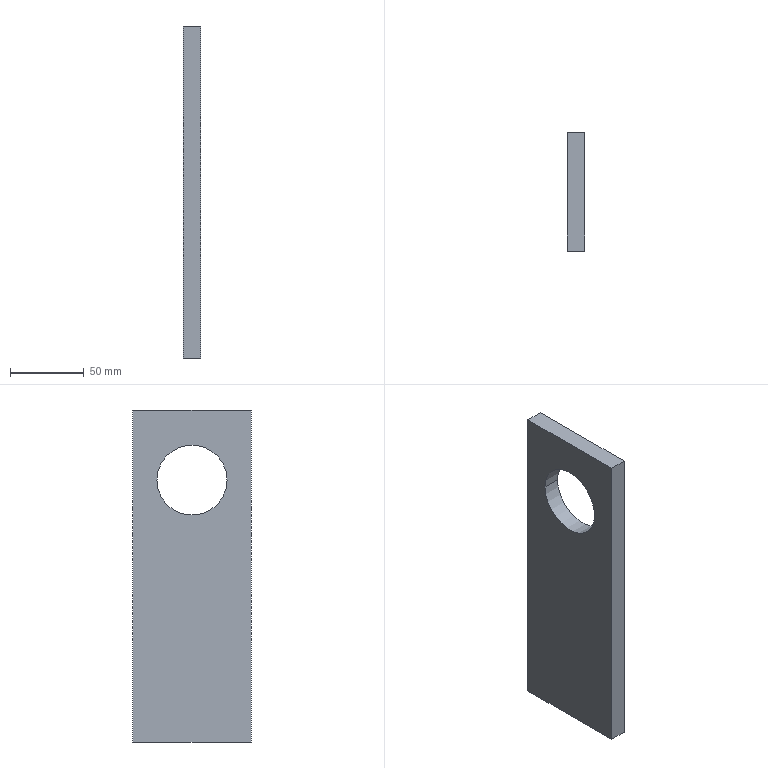Part | STEP file | 2026.6.15-Main Assembly图.sldasm-Part-143 | 1 solid | 32 faces | box 12 x 80.5 x 225 mm | volume 195559 mm3 | cone 16 | cylinder 10 | plane 6 | commonest cylinder face diameters 4.2 x8 47.5 x2
STEP:
#1=CARTESIAN_POINT('',(-1492.124,577.531,4275.837));
#2=VERTEX_POINT('',#1);
#3=CARTESIAN_POINT('',(-1492.124,581.731,4275.837));
#4=VERTEX_POINT('',#3);
#5=CARTESIAN_POINT('',(-1492.124,579.631,4275.837));
#6=DIRECTION('',(1.,0.,0.));
#7=DIRECTION('',(0.,1.,0.));
#8=AXIS2_PLACEMENT_3D('',#5,#6,#7);
#9=CIRCLE('',#8,2.1);
#10=EDGE_CURVE('',#2,#4,#9,.T.);
#11=ORIENTED_EDGE('',*,*,#10,.F.);
#12=CARTESIAN_POINT('',(-1491.724,577.131,4275.837));
#13=VERTEX_POINT('',#12);
#14=CARTESIAN_POINT('',(-1491.724,577.131,4275.837));
#15=DIRECTION('',(0.7071,-0.7071,0.));
#16=VECTOR('',#15,1000.);
#17=LINE('',#14,#16);
#18=EDGE_CURVE('',#2,#13,#17,.T.);
#19=ORIENTED_EDGE('',*,*,#18,.T.);
#20=CARTESIAN_POINT('',(-1491.724,582.131,4275.837));
#21=VERTEX_POINT('',#20);
#22=CARTESIAN_POINT('',(-1491.724,579.631,4275.837));
#23=DIRECTION('',(-1.,0.,0.));
#24=DIRECTION('',(0.,1.,0.));
#25=AXIS2_PLACEMENT_3D('',#22,#23,#24);
#26=CIRCLE('',#25,2.5);
#27=EDGE_CURVE('',#21,#13,#26,.T.);
#28=ORIENTED_EDGE('',*,*,#27,.F.);
#29=CARTESIAN_POINT('',(-1491.724,582.131,4275.837));
#30=DIRECTION('',(0.7071,0.7071,0.));
#31=VECTOR('',#30,1000.);
#32=LINE('',#29,#31);
#33=EDGE_CURVE('',#4,#21,#32,.T.);
#34=ORIENTED_EDGE('',*,*,#33,.F.);
#35=EDGE_LOOP('',(#11,#19,#28,#34));
#36=FACE_OUTER_BOUND('',#35,.T.);
#37=CARTESIAN_POINT('',(-1491.724,579.631,4275.837));
#38=DIRECTION('',(1.,0.,0.));
#39=DIRECTION('',(0.,1.,0.));
#40=AXIS2_PLACEMENT_3D('',#37,#38,#39);
#41=CONICAL_SURFACE('',#40,2.5,0.7854);
#42=ADVANCED_FACE('',(#36),#41,.F.);
#43=ORIENTED_EDGE('',*,*,#10,.T.);
#44=CARTESIAN_POINT('',(-1500.724,581.731,4275.837));
#45=VERTEX_POINT('',#44);
#46=CARTESIAN_POINT('',(-1491.724,581.731,4275.837));
#47=DIRECTION('',(-1.,0.,0.));
#48=VECTOR('',#47,1000.);
#49=LINE('',#46,#48);
#50=EDGE_CURVE('',#4,#45,#49,.T.);
#51=ORIENTED_EDGE('',*,*,#50,.T.);
#52=CARTESIAN_POINT('',(-1500.724,577.531,4275.837));
#53=VERTEX_POINT('',#52);
#54=CARTESIAN_POINT('',(-1500.724,579.631,4275.837));
#55=DIRECTION('',(1.,0.,0.));
#56=DIRECTION('',(0.,-1.,0.));
#57=AXIS2_PLACEMENT_3D('',#54,#55,#56);
#58=CIRCLE('',#57,2.1);
#59=EDGE_CURVE('',#53,#45,#58,.T.);
#60=ORIENTED_EDGE('',*,*,#59,.F.);
#61=CARTESIAN_POINT('',(-1491.724,577.531,4275.837));
#62=DIRECTION('',(-1.,0.,0.));
#63=VECTOR('',#62,1000.);
#64=LINE('',#61,#63);
#65=EDGE_CURVE('',#2,#53,#64,.T.);
#66=ORIENTED_EDGE('',*,*,#65,.F.);
#67=EDGE_LOOP('',(#43,#51,#60,#66));
#68=FACE_OUTER_BOUND('',#67,.T.);
#69=CARTESIAN_POINT('',(-1491.724,579.631,4275.837));
#70=DIRECTION('',(-1.,0.,0.));
#71=DIRECTION('',(0.,-1.,0.));
#72=AXIS2_PLACEMENT_3D('',#69,#70,#71);
#73=CYLINDRICAL_SURFACE('',#72,2.1);
#74=ADVANCED_FACE('',(#68),#73,.F.);
#75=CARTESIAN_POINT('',(-1501.986,579.631,4275.837));
#76=VERTEX_POINT('',#75);
#77=CARTESIAN_POINT('',(-1500.724,581.731,4275.837));
#78=DIRECTION('',(0.515,0.8572,0.));
#79=VECTOR('',#78,1000.);
#80=LINE('',#77,#79);
#81=EDGE_CURVE('',#76,#45,#80,.T.);
#82=ORIENTED_EDGE('',*,*,#81,.F.);
#83=CARTESIAN_POINT('',(-1500.724,577.531,4275.837));
#84=DIRECTION('',(0.515,-0.8572,0.));
#85=VECTOR('',#84,1000.);
#86=LINE('',#83,#85);
#87=EDGE_CURVE('',#76,#53,#86,.T.);
#88=ORIENTED_EDGE('',*,*,#87,.T.);
#89=ORIENTED_EDGE('',*,*,#59,.T.);
#90=EDGE_LOOP('',(#82,#88,#89));
#91=FACE_OUTER_BOUND('',#90,.T.);
#92=CARTESIAN_POINT('',(-1500.724,579.631,4275.837));
#93=DIRECTION('',(1.,0.,0.));
#94=DIRECTION('',(0.,1.,0.));
#95=AXIS2_PLACEMENT_3D('',#92,#93,#94);
#96=CONICAL_SURFACE('',#95,2.1,1.03);
#97=ADVANCED_FACE('',(#91),#96,.F.);
#98=CARTESIAN_POINT('',(-1492.124,577.531,4316.496));
#99=VERTEX_POINT('',#98);
#100=CARTESIAN_POINT('',(-1492.124,581.731,4316.496));
#101=VERTEX_POINT('',#100);
#102=CARTESIAN_POINT('',(-1492.124,579.631,4316.496));
#103=DIRECTION('',(1.,0.,0.));
#104=DIRECTION('',(0.,1.,0.));
#105=AXIS2_PLACEMENT_3D('',#102,#103,#104);
#106=CIRCLE('',#105,2.1);
#107=EDGE_CURVE('',#99,#101,#106,.T.);
#108=ORIENTED_EDGE('',*,*,#107,.F.);
#109=CARTESIAN_POINT('',(-1491.724,577.131,4316.496));
#110=VERTEX_POINT('',#109);
#111=CARTESIAN_POINT('',(-1491.724,577.131,4316.496));
#112=DIRECTION('',(0.7071,-0.7071,0.));
#113=VECTOR('',#112,1000.);
#114=LINE('',#111,#113);
#115=EDGE_CURVE('',#99,#110,#114,.T.);
#116=ORIENTED_EDGE('',*,*,#115,.T.);
#117=CARTESIAN_POINT('',(-1491.724,582.131,4316.496));
#118=VERTEX_POINT('',#117);
#119=CARTESIAN_POINT('',(-1491.724,579.631,4316.496));
#120=DIRECTION('',(-1.,0.,0.));
#121=DIRECTION('',(0.,1.,0.));
#122=AXIS2_PLACEMENT_3D('',#119,#120,#121);
#123=CIRCLE('',#122,2.5);
#124=EDGE_CURVE('',#118,#110,#123,.T.);
#125=ORIENTED_EDGE('',*,*,#124,.F.);
#126=CARTESIAN_POINT('',(-1491.724,582.131,4316.496));
#127=DIRECTION('',(0.7071,0.7071,0.));
#128=VECTOR('',#127,1000.);
#129=LINE('',#126,#128);
#130=EDGE_CURVE('',#101,#118,#129,.T.);
#131=ORIENTED_EDGE('',*,*,#130,.F.);
#132=EDGE_LOOP('',(#108,#116,#125,#131));
#133=FACE_OUTER_BOUND('',#132,.T.);
#134=CARTESIAN_POINT('',(-1491.724,579.631,4316.496));
#135=DIRECTION('',(1.,0.,0.));
#136=DIRECTION('',(0.,1.,0.));
#137=AXIS2_PLACEMENT_3D('',#134,#135,#136);
#138=CONICAL_SURFACE('',#137,2.5,0.7854);
#139=ADVANCED_FACE('',(#133),#138,.F.);
#140=ORIENTED_EDGE('',*,*,#107,.T.);
#141=CARTESIAN_POINT('',(-1500.724,581.731,4316.496));
#142=VERTEX_POINT('',#141);
#143=CARTESIAN_POINT('',(-1491.724,581.731,4316.496));
#144=DIRECTION('',(-1.,0.,0.));
#145=VECTOR('',#144,1000.);
#146=LINE('',#143,#145);
#147=EDGE_CURVE('',#101,#142,#146,.T.);
#148=ORIENTED_EDGE('',*,*,#147,.T.);
#149=CARTESIAN_POINT('',(-1500.724,577.531,4316.496));
#150=VERTEX_POINT('',#149);
#151=CARTESIAN_POINT('',(-1500.724,579.631,4316.496));
#152=DIRECTION('',(1.,0.,0.));
#153=DIRECTION('',(0.,-1.,0.));
#154=AXIS2_PLACEMENT_3D('',#151,#152,#153);
#155=CIRCLE('',#154,2.1);
#156=EDGE_CURVE('',#150,#142,#155,.T.);
#157=ORIENTED_EDGE('',*,*,#156,.F.);
#158=CARTESIAN_POINT('',(-1491.724,577.531,4316.496));
#159=DIRECTION('',(-1.,0.,0.));
#160=VECTOR('',#159,1000.);
#161=LINE('',#158,#160);
#162=EDGE_CURVE('',#99,#150,#161,.T.);
#163=ORIENTED_EDGE('',*,*,#162,.F.);
#164=EDGE_LOOP('',(#140,#148,#157,#163));
#165=FACE_OUTER_BOUND('',#164,.T.);
#166=CARTESIAN_POINT('',(-1491.724,579.631,4316.496));
#167=DIRECTION('',(-1.,0.,0.));
#168=DIRECTION('',(0.,-1.,0.));
#169=AXIS2_PLACEMENT_3D('',#166,#167,#168);
#170=CYLINDRICAL_SURFACE('',#169,2.1);
#171=ADVANCED_FACE('',(#165),#170,.F.);
#172=CARTESIAN_POINT('',(-1501.986,579.631,4316.496));
#173=VERTEX_POINT('',#172);
#174=CARTESIAN_POINT('',(-1500.724,581.731,4316.496));
#175=DIRECTION('',(0.515,0.8572,0.));
#176=VECTOR('',#175,1000.);
#177=LINE('',#174,#176);
#178=EDGE_CURVE('',#173,#142,#177,.T.);
#179=ORIENTED_EDGE('',*,*,#178,.F.);
#180=CARTESIAN_POINT('',(-1500.724,577.531,4316.496));
#181=DIRECTION('',(0.515,-0.8572,0.));
#182=VECTOR('',#181,1000.);
#183=LINE('',#180,#182);
#184=EDGE_CURVE('',#173,#150,#183,.T.);
#185=ORIENTED_EDGE('',*,*,#184,.T.);
#186=ORIENTED_EDGE('',*,*,#156,.T.);
#187=EDGE_LOOP('',(#179,#185,#186));
#188=FACE_OUTER_BOUND('',#187,.T.);
#189=CARTESIAN_POINT('',(-1500.724,579.631,4316.496));
#190=DIRECTION('',(1.,0.,0.));
#191=DIRECTION('',(0.,1.,0.));
#192=AXIS2_PLACEMENT_3D('',#189,#190,#191);
#193=CONICAL_SURFACE('',#192,2.1,1.03);
#194=ADVANCED_FACE('',(#188),#193,.F.);
#195=CARTESIAN_POINT('',(-1492.124,536.872,4316.496));
#196=VERTEX_POINT('',#195);
#197=CARTESIAN_POINT('',(-1492.124,541.072,4316.496));
#198=VERTEX_POINT('',#197);
#199=CARTESIAN_POINT('',(-1492.124,538.972,4316.496));
#200=DIRECTION('',(1.,0.,0.));
#201=DIRECTION('',(0.,1.,0.));
#202=AXIS2_PLACEMENT_3D('',#199,#200,#201);
#203=CIRCLE('',#202,2.1);
#204=EDGE_CURVE('',#196,#198,#203,.T.);
#205=ORIENTED_EDGE('',*,*,#204,.F.);
#206=CARTESIAN_POINT('',(-1491.724,536.472,4316.496));
#207=VERTEX_POINT('',#206);
#208=CARTESIAN_POINT('',(-1491.724,536.472,4316.496));
#209=DIRECTION('',(0.7071,-0.7071,0.));
#210=VECTOR('',#209,1000.);
#211=LINE('',#208,#210);
#212=EDGE_CURVE('',#196,#207,#211,.T.);
#213=ORIENTED_EDGE('',*,*,#212,.T.);
#214=CARTESIAN_POINT('',(-1491.724,541.472,4316.496));
#215=VERTEX_POINT('',#214);
#216=CARTESIAN_POINT('',(-1491.724,538.972,4316.496));
#217=DIRECTION('',(-1.,0.,0.));
#218=DIRECTION('',(0.,1.,0.));
#219=AXIS2_PLACEMENT_3D('',#216,#217,#218);
#220=CIRCLE('',#219,2.5);
#221=EDGE_CURVE('',#215,#207,#220,.T.);
#222=ORIENTED_EDGE('',*,*,#221,.F.);
#223=CARTESIAN_POINT('',(-1491.724,541.472,4316.496));
#224=DIRECTION('',(0.7071,0.7071,0.));
#225=VECTOR('',#224,1000.);
#226=LINE('',#223,#225);
#227=EDGE_CURVE('',#198,#215,#226,.T.);
#228=ORIENTED_EDGE('',*,*,#227,.F.);
#229=EDGE_LOOP('',(#205,#213,#222,#228));
#230=FACE_OUTER_BOUND('',#229,.T.);
#231=CARTESIAN_POINT('',(-1491.724,538.972,4316.496));
#232=DIRECTION('',(1.,0.,0.));
#233=DIRECTION('',(0.,1.,0.));
#234=AXIS2_PLACEMENT_3D('',#231,#232,#233);
#235=CONICAL_SURFACE('',#234,2.5,0.7854);
#236=ADVANCED_FACE('',(#230),#235,.F.);
#237=ORIENTED_EDGE('',*,*,#204,.T.);
#238=CARTESIAN_POINT('',(-1500.724,541.072,4316.496));
#239=VERTEX_POINT('',#238);
#240=CARTESIAN_POINT('',(-1491.724,541.072,4316.496));
#241=DIRECTION('',(-1.,0.,0.));
#242=VECTOR('',#241,1000.);
#243=LINE('',#240,#242);
#244=EDGE_CURVE('',#198,#239,#243,.T.);
#245=ORIENTED_EDGE('',*,*,#244,.T.);
#246=CARTESIAN_POINT('',(-1500.724,536.872,4316.496));
#247=VERTEX_POINT('',#246);
#248=CARTESIAN_POINT('',(-1500.724,538.972,4316.496));
#249=DIRECTION('',(1.,0.,0.));
#250=DIRECTION('',(0.,-1.,0.));
#251=AXIS2_PLACEMENT_3D('',#248,#249,#250);
#252=CIRCLE('',#251,2.1);
#253=EDGE_CURVE('',#247,#239,#252,.T.);
#254=ORIENTED_EDGE('',*,*,#253,.F.);
#255=CARTESIAN_POINT('',(-1491.724,536.872,4316.496));
#256=DIRECTION('',(-1.,0.,0.));
#257=VECTOR('',#256,1000.);
#258=LINE('',#255,#257);
#259=EDGE_CURVE('',#196,#247,#258,.T.);
#260=ORIENTED_EDGE('',*,*,#259,.F.);
#261=EDGE_LOOP('',(#237,#245,#254,#260));
#262=FACE_OUTER_BOUND('',#261,.T.);
#263=CARTESIAN_POINT('',(-1491.724,538.972,4316.496));
#264=DIRECTION('',(-1.,0.,0.));
#265=DIRECTION('',(0.,-1.,0.));
#266=AXIS2_PLACEMENT_3D('',#263,#264,#265);
#267=CYLINDRICAL_SURFACE('',#266,2.1);
#268=ADVANCED_FACE('',(#262),#267,.F.);
#269=CARTESIAN_POINT('',(-1501.986,538.972,4316.496));
#270=VERTEX_POINT('',#269);
#271=CARTESIAN_POINT('',(-1500.724,541.072,4316.496));
#272=DIRECTION('',(0.515,0.8572,0.));
#273=VECTOR('',#272,1000.);
#274=LINE('',#271,#273);
#275=EDGE_CURVE('',#270,#239,#274,.T.);
#276=ORIENTED_EDGE('',*,*,#275,.F.);
#277=CARTESIAN_POINT('',(-1500.724,536.872,4316.496));
#278=DIRECTION('',(0.515,-0.8572,0.));
#279=VECTOR('',#278,1000.);
#280=LINE('',#277,#279);
#281=EDGE_CURVE('',#270,#247,#280,.T.);
#282=ORIENTED_EDGE('',*,*,#281,.T.);
#283=ORIENTED_EDGE('',*,*,#253,.T.);
#284=EDGE_LOOP('',(#276,#282,#283));
#285=FACE_OUTER_BOUND('',#284,.T.);
#286=CARTESIAN_POINT('',(-1500.724,538.972,4316.496));
#287=DIRECTION('',(1.,0.,0.));
#288=DIRECTION('',(0.,1.,0.));
#289=AXIS2_PLACEMENT_3D('',#286,#287,#288);
#290=CONICAL_SURFACE('',#289,2.1,1.03);
#291=ADVANCED_FACE('',(#285),#290,.F.);
#292=CARTESIAN_POINT('',(-1492.124,536.872,4275.837));
#293=VERTEX_POINT('',#292);
#294=CARTESIAN_POINT('',(-1492.124,541.072,4275.837));
#295=VERTEX_POINT('',#294);
#296=CARTESIAN_POINT('',(-1492.124,538.972,4275.837));
#297=DIRECTION('',(1.,0.,0.));
#298=DIRECTION('',(0.,1.,0.));
#299=AXIS2_PLACEMENT_3D('',#296,#297,#298);
#300=CIRCLE('',#299,2.1);
#301=EDGE_CURVE('',#293,#295,#300,.T.);
#302=ORIENTED_EDGE('',*,*,#301,.F.);
#303=CARTESIAN_POINT('',(-1491.724,536.472,4275.837));
#304=VERTEX_POINT('',#303);
#305=CARTESIAN_POINT('',(-1491.724,536.472,4275.837));
#306=DIRECTION('',(0.7071,-0.7071,0.));
#307=VECTOR('',#306,1000.);
#308=LINE('',#305,#307);
#309=EDGE_CURVE('',#293,#304,#308,.T.);
#310=ORIENTED_EDGE('',*,*,#309,.T.);
#311=CARTESIAN_POINT('',(-1491.724,541.472,4275.837));
#312=VERTEX_POINT('',#311);
#313=CARTESIAN_POINT('',(-1491.724,538.972,4275.837));
#314=DIRECTION('',(-1.,0.,0.));
#315=DIRECTION('',(0.,1.,0.));
#316=AXIS2_PLACEMENT_3D('',#313,#314,#315);
#317=CIRCLE('',#316,2.5);
#318=EDGE_CURVE('',#312,#304,#317,.T.);
#319=ORIENTED_EDGE('',*,*,#318,.F.);
#320=CARTESIAN_POINT('',(-1491.724,541.472,4275.837));
#321=DIRECTION('',(0.7071,0.7071,0.));
#322=VECTOR('',#321,1000.);
#323=LINE('',#320,#322);
#324=EDGE_CURVE('',#295,#312,#323,.T.);
#325=ORIENTED_EDGE('',*,*,#324,.F.);
#326=EDGE_LOOP('',(#302,#310,#319,#325));
#327=FACE_OUTER_BOUND('',#326,.T.);
#328=CARTESIAN_POINT('',(-1491.724,538.972,4275.837));
#329=DIRECTION('',(1.,0.,0.));
#330=DIRECTION('',(0.,1.,0.));
#331=AXIS2_PLACEMENT_3D('',#328,#329,#330);
#332=CONICAL_SURFACE('',#331,2.5,0.7854);
#333=ADVANCED_FACE('',(#327),#332,.F.);
#334=ORIENTED_EDGE('',*,*,#301,.T.);
#335=CARTESIAN_POINT('',(-1500.724,541.072,4275.837));
#336=VERTEX_POINT('',#335);
#337=CARTESIAN_POINT('',(-1491.724,541.072,4275.837));
#338=DIRECTION('',(-1.,0.,0.));
#339=VECTOR('',#338,1000.);
#340=LINE('',#337,#339);
#341=EDGE_CURVE('',#295,#336,#340,.T.);
#342=ORIENTED_EDGE('',*,*,#341,.T.);
#343=CARTESIAN_POINT('',(-1500.724,536.872,4275.837));
#344=VERTEX_POINT('',#343);
#345=CARTESIAN_POINT('',(-1500.724,538.972,4275.837));
#346=DIRECTION('',(1.,0.,0.));
#347=DIRECTION('',(0.,-1.,0.));
#348=AXIS2_PLACEMENT_3D('',#345,#346,#347);
#349=CIRCLE('',#348,2.1);
#350=EDGE_CURVE('',#344,#336,#349,.T.);
#351=ORIENTED_EDGE('',*,*,#350,.F.);
#352=CARTESIAN_POINT('',(-1491.724,536.872,4275.837));
#353=DIRECTION('',(-1.,0.,0.));
#354=VECTOR('',#353,1000.);
#355=LINE('',#352,#354);
#356=EDGE_CURVE('',#293,#344,#355,.T.);
#357=ORIENTED_EDGE('',*,*,#356,.F.);
#358=EDGE_LOOP('',(#334,#342,#351,#357));
#359=FACE_OUTER_BOUND('',#358,.T.);
#360=CARTESIAN_POINT('',(-1491.724,538.972,4275.837));
#361=DIRECTION('',(-1.,0.,0.));
#362=DIRECTION('',(0.,-1.,0.));
#363=AXIS2_PLACEMENT_3D('',#360,#361,#362);
#364=CYLINDRICAL_SURFACE('',#363,2.1);
#365=ADVANCED_FACE('',(#359),#364,.F.);
#366=CARTESIAN_POINT('',(-1501.986,538.972,4275.837));
#367=VERTEX_POINT('',#366);
#368=CARTESIAN_POINT('',(-1500.724,541.072,4275.837));
#369=DIRECTION('',(0.515,0.8572,0.));
#370=VECTOR('',#369,1000.);
#371=LINE('',#368,#370);
#372=EDGE_CURVE('',#367,#336,#371,.T.);
#373=ORIENTED_EDGE('',*,*,#372,.F.);
#374=CARTESIAN_POINT('',(-1500.724,536.872,4275.837));
#375=DIRECTION('',(0.515,-0.8572,0.));
#376=VECTOR('',#375,1000.);
#377=LINE('',#374,#376);
#378=EDGE_CURVE('',#367,#344,#377,.T.);
#379=ORIENTED_EDGE('',*,*,#378,.T.);
#380=ORIENTED_EDGE('',*,*,#350,.T.);
#381=EDGE_LOOP('',(#373,#379,#380));
#382=FACE_OUTER_BOUND('',#381,.T.);
#383=CARTESIAN_POINT('',(-1500.724,538.972,4275.837));
#384=DIRECTION('',(1.,0.,0.));
#385=DIRECTION('',(0.,1.,0.));
#386=AXIS2_PLACEMENT_3D('',#383,#384,#385);
#387=CONICAL_SURFACE('',#386,2.1,1.03);
#388=ADVANCED_FACE('',(#382),#387,.F.);
#389=CARTESIAN_POINT('',(-1503.724,535.551,4296.167));
#390=VERTEX_POINT('',#389);
#391=CARTESIAN_POINT('',(-1503.724,583.051,4296.167));
#392=VERTEX_POINT('',#391);
#393=CARTESIAN_POINT('',(-1503.724,559.301,4296.167));
#394=DIRECTION('',(1.,0.,0.));
#395=DIRECTION('',(0.,1.,0.));
#396=AXIS2_PLACEMENT_3D('',#393,#394,#395);
#397=CIRCLE('',#396,23.75);
#398=EDGE_CURVE('',#390,#392,#397,.T.);
#399=ORIENTED_EDGE('',*,*,#398,.F.);
#400=CARTESIAN_POINT('',(-1491.724,535.551,4296.167));
#401=VERTEX_POINT('',#400);
#402=CARTESIAN_POINT('',(-1503.724,535.551,4296.167));
#403=DIRECTION('',(1.,0.,0.));
#404=VECTOR('',#403,1000.);
#405=LINE('',#402,#404);
#406=EDGE_CURVE('',#390,#401,#405,.T.);
#407=ORIENTED_EDGE('',*,*,#406,.T.);
#408=CARTESIAN_POINT('',(-1491.724,583.051,4296.167));
#409=VERTEX_POINT('',#408);
#410=CARTESIAN_POINT('',(-1491.724,559.301,4296.167));
#411=DIRECTION('',(1.,0.,0.));
#412=DIRECTION('',(0.,1.,0.));
#413=AXIS2_PLACEMENT_3D('',#410,#411,#412);
#414=CIRCLE('',#413,23.75);
#415=EDGE_CURVE('',#401,#409,#414,.T.);
#416=ORIENTED_EDGE('',*,*,#415,.T.);
#417=CARTESIAN_POINT('',(-1503.724,583.051,4296.167));
#418=DIRECTION('',(1.,0.,0.));
#419=VECTOR('',#418,1000.);
#420=LINE('',#417,#419);
#421=EDGE_CURVE('',#392,#409,#420,.T.);
#422=ORIENTED_EDGE('',*,*,#421,.F.);
#423=EDGE_LOOP('',(#399,#407,#416,#422));
#424=FACE_OUTER_BOUND('',#423,.T.);
#425=CARTESIAN_POINT('',(-1503.724,559.301,4296.167));
#426=DIRECTION('',(1.,0.,0.));
#427=DIRECTION('',(0.,1.,0.));
#428=AXIS2_PLACEMENT_3D('',#425,#426,#427);
#429=CYLINDRICAL_SURFACE('',#428,23.75);
#430=ADVANCED_FACE('',(#424),#429,.F.);
#431=CARTESIAN_POINT('',(-1491.724,519.051,4343.667));
#432=VERTEX_POINT('',#431);
#433=CARTESIAN_POINT('',(-1491.724,519.051,4118.667));
#434=VERTEX_POINT('',#433);
#435=CARTESIAN_POINT('',(-1491.724,519.051,4343.667));
#436=DIRECTION('',(0.,0.,-1.));
#437=VECTOR('',#436,1000.);
#438=LINE('',#435,#437);
#439=EDGE_CURVE('',#432,#434,#438,.T.);
#440=ORIENTED_EDGE('',*,*,#439,.F.);
#441=CARTESIAN_POINT('',(-1503.724,519.051,4343.667));
#442=VERTEX_POINT('',#441);
#443=CARTESIAN_POINT('',(-1503.724,519.051,4343.667));
#444=DIRECTION('',(1.,0.,0.));
#445=VECTOR('',#444,1000.);
#446=LINE('',#443,#445);
#447=EDGE_CURVE('',#442,#432,#446,.T.);
#448=ORIENTED_EDGE('',*,*,#447,.F.);
#449=CARTESIAN_POINT('',(-1503.724,519.051,4118.667));
#450=VERTEX_POINT('',#449);
#451=CARTESIAN_POINT('',(-1503.724,519.051,4343.667));
#452=DIRECTION('',(0.,0.,-1.));
#453=VECTOR('',#452,1000.);
#454=LINE('',#451,#453);
#455=EDGE_CURVE('',#442,#450,#454,.T.);
#456=ORIENTED_EDGE('',*,*,#455,.T.);
#457=CARTESIAN_POINT('',(-1503.724,519.051,4118.667));
#458=DIRECTION('',(1.,0.,0.));
#459=VECTOR('',#458,1000.);
#460=LINE('',#457,#459);
#461=EDGE_CURVE('',#450,#434,#460,.T.);
#462=ORIENTED_EDGE('',*,*,#461,.T.);
#463=EDGE_LOOP('',(#440,#448,#456,#462));
#464=FACE_OUTER_BOUND('',#463,.T.);
#465=CARTESIAN_POINT('',(-1503.724,519.051,4343.667));
#466=DIRECTION('',(0.,-1.,0.));
#467=DIRECTION('',(0.,0.,-1.));
#468=AXIS2_PLACEMENT_3D('',#465,#466,#467);
#469=PLANE('',#468);
#470=ADVANCED_FACE('',(#464),#469,.T.);
#471=CARTESIAN_POINT('',(-1491.724,599.551,4118.667));
#472=VERTEX_POINT('',#471);
#473=CARTESIAN_POINT('',(-1491.724,519.051,4118.667));
#474=DIRECTION('',(0.,1.,0.));
#475=VECTOR('',#474,1000.);
#476=LINE('',#473,#475);
#477=EDGE_CURVE('',#434,#472,#476,.T.);
#478=ORIENTED_EDGE('',*,*,#477,.F.);
#479=ORIENTED_EDGE('',*,*,#461,.F.);
#480=CARTESIAN_POINT('',(-1503.724,599.551,4118.667));
#481=VERTEX_POINT('',#480);
#482=CARTESIAN_POINT('',(-1503.724,519.051,4118.667));
#483=DIRECTION('',(0.,1.,0.));
#484=VECTOR('',#483,1000.);
#485=LINE('',#482,#484);
#486=EDGE_CURVE('',#450,#481,#485,.T.);
#487=ORIENTED_EDGE('',*,*,#486,.T.);
#488=CARTESIAN_POINT('',(-1503.724,599.551,4118.667));
#489=DIRECTION('',(1.,0.,0.));
#490=VECTOR('',#489,1000.);
#491=LINE('',#488,#490);
#492=EDGE_CURVE('',#481,#472,#491,.T.);
#493=ORIENTED_EDGE('',*,*,#492,.T.);
#494=EDGE_LOOP('',(#478,#479,#487,#493));
#495=FACE_OUTER_BOUND('',#494,.T.);
#496=CARTESIAN_POINT('',(-1503.724,519.051,4118.667));
#497=DIRECTION('',(0.,0.,-1.));
#498=DIRECTION('',(0.,1.,0.));
#499=AXIS2_PLACEMENT_3D('',#496,#497,#498);
#500=PLANE('',#499);
#501=ADVANCED_FACE('',(#495),#500,.T.);
#502=CARTESIAN_POINT('',(-1491.724,599.551,4343.667));
#503=VERTEX_POINT('',#502);
#504=CARTESIAN_POINT('',(-1491.724,599.551,4118.667));
#505=DIRECTION('',(0.,0.,1.));
#506=VECTOR('',#505,1000.);
#507=LINE('',#504,#506);
#508=EDGE_CURVE('',#472,#503,#507,.T.);
#509=ORIENTED_EDGE('',*,*,#508,.F.);
#510=ORIENTED_EDGE('',*,*,#492,.F.);
#511=CARTESIAN_POINT('',(-1503.724,599.551,4343.667));
#512=VERTEX_POINT('',#511);
#513=CARTESIAN_POINT('',(-1503.724,599.551,4118.667));
#514=DIRECTION('',(0.,0.,1.));
#515=VECTOR('',#514,1000.);
#516=LINE('',#513,#515);
#517=EDGE_CURVE('',#481,#512,#516,.T.);
#518=ORIENTED_EDGE('',*,*,#517,.T.);
#519=CARTESIAN_POINT('',(-1503.724,599.551,4343.667));
#520=DIRECTION('',(1.,0.,0.));
#521=VECTOR('',#520,1000.);
#522=LINE('',#519,#521);
#523=EDGE_CURVE('',#512,#503,#522,.T.);
#524=ORIENTED_EDGE('',*,*,#523,.T.);
#525=EDGE_LOOP('',(#509,#510,#518,#524));
#526=FACE_OUTER_BOUND('',#525,.T.);
#527=CARTESIAN_POINT('',(-1503.724,599.551,4118.667));
#528=DIRECTION('',(0.,1.,0.));
#529=DIRECTION('',(0.,0.,1.));
#530=AXIS2_PLACEMENT_3D('',#527,#528,#529);
#531=PLANE('',#530);
#532=ADVANCED_FACE('',(#526),#531,.T.);
#533=CARTESIAN_POINT('',(-1491.724,599.551,4343.667));
#534=DIRECTION('',(0.,-1.,0.));
#535=VECTOR('',#534,1000.);
#536=LINE('',#533,#535);
#537=EDGE_CURVE('',#503,#432,#536,.T.);
#538=ORIENTED_EDGE('',*,*,#537,.F.);
#539=ORIENTED_EDGE('',*,*,#523,.F.);
#540=CARTESIAN_POINT('',(-1503.724,599.551,4343.667));
#541=DIRECTION('',(0.,-1.,0.));
#542=VECTOR('',#541,1000.);
#543=LINE('',#540,#542);
#544=EDGE_CURVE('',#512,#442,#543,.T.);
#545=ORIENTED_EDGE('',*,*,#544,.T.);
#546=ORIENTED_EDGE('',*,*,#447,.T.);
#547=EDGE_LOOP('',(#538,#539,#545,#546));
#548=FACE_OUTER_BOUND('',#547,.T.);
#549=CARTESIAN_POINT('',(-1503.724,599.551,4343.667));
#550=DIRECTION('',(0.,0.,1.));
#551=DIRECTION('',(0.,-1.,0.));
#552=AXIS2_PLACEMENT_3D('',#549,#550,#551);
#553=PLANE('',#552);
#554=ADVANCED_FACE('',(#548),#553,.T.);
#555=ORIENTED_EDGE('',*,*,#406,.F.);
#556=CARTESIAN_POINT('',(-1503.724,559.301,4296.167));
#557=DIRECTION('',(1.,0.,0.));
#558=DIRECTION('',(0.,1.,0.));
#559=AXIS2_PLACEMENT_3D('',#556,#557,#558);
#560=CIRCLE('',#559,23.75);
#561=EDGE_CURVE('',#392,#390,#560,.T.);
#562=ORIENTED_EDGE('',*,*,#561,.F.);
#563=ORIENTED_EDGE('',*,*,#421,.T.);
#564=CARTESIAN_POINT('',(-1491.724,559.301,4296.167));
#565=DIRECTION('',(1.,0.,0.));
#566=DIRECTION('',(0.,1.,0.));
#567=AXIS2_PLACEMENT_3D('',#564,#565,#566);
#568=CIRCLE('',#567,23.75);
#569=EDGE_CURVE('',#409,#401,#568,.T.);
#570=ORIENTED_EDGE('',*,*,#569,.T.);
#571=EDGE_LOOP('',(#555,#562,#563,#570));
#572=FACE_OUTER_BOUND('',#571,.T.);
#573=CARTESIAN_POINT('',(-1503.724,559.301,4296.167));
#574=DIRECTION('',(1.,0.,0.));
#575=DIRECTION('',(0.,1.,0.));
#576=AXIS2_PLACEMENT_3D('',#573,#574,#575);
#577=CYLINDRICAL_SURFACE('',#576,23.75);
#578=ADVANCED_FACE('',(#572),#577,.F.);
#579=ORIENTED_EDGE('',*,*,#455,.F.);
#580=ORIENTED_EDGE('',*,*,#544,.F.);
#581=ORIENTED_EDGE('',*,*,#517,.F.);
#582=ORIENTED_EDGE('',*,*,#486,.F.);
#583=EDGE_LOOP('',(#579,#580,#581,#582));
#584=FACE_OUTER_BOUND('',#583,.T.);
#585=ORIENTED_EDGE('',*,*,#561,.T.);
#586=ORIENTED_EDGE('',*,*,#398,.T.);
#587=EDGE_LOOP('',(#585,#586));
#588=FACE_BOUND('',#587,.T.);
#589=CARTESIAN_POINT('',(-1503.724,559.301,4296.167));
#590=DIRECTION('',(1.,0.,0.));
#591=DIRECTION('',(0.,1.,0.));
#592=AXIS2_PLACEMENT_3D('',#589,#590,#591);
#593=PLANE('',#592);
#594=ADVANCED_FACE('',(#584,#588),#593,.F.);
#595=ORIENTED_EDGE('',*,*,#27,.T.);
#596=CARTESIAN_POINT('',(-1491.724,579.631,4275.837));
#597=DIRECTION('',(-1.,0.,0.));
#598=DIRECTION('',(0.,1.,0.));
#599=AXIS2_PLACEMENT_3D('',#596,#597,#598);
#600=CIRCLE('',#599,2.5);
#601=EDGE_CURVE('',#13,#21,#600,.T.);
#602=ORIENTED_EDGE('',*,*,#601,.T.);
#603=EDGE_LOOP('',(#595,#602));
#604=FACE_BOUND('',#603,.T.);
#605=ORIENTED_EDGE('',*,*,#124,.T.);
#606=CARTESIAN_POINT('',(-1491.724,579.631,4316.496));
#607=DIRECTION('',(-1.,0.,0.));
#608=DIRECTION('',(0.,1.,0.));
#609=AXIS2_PLACEMENT_3D('',#606,#607,#608);
#610=CIRCLE('',#609,2.5);
#611=EDGE_CURVE('',#110,#118,#610,.T.);
#612=ORIENTED_EDGE('',*,*,#611,.T.);
#613=EDGE_LOOP('',(#605,#612));
#614=FACE_BOUND('',#613,.T.);
#615=ORIENTED_EDGE('',*,*,#221,.T.);
#616=CARTESIAN_POINT('',(-1491.724,538.972,4316.496));
#617=DIRECTION('',(-1.,0.,0.));
#618=DIRECTION('',(0.,1.,0.));
#619=AXIS2_PLACEMENT_3D('',#616,#617,#618);
#620=CIRCLE('',#619,2.5);
#621=EDGE_CURVE('',#207,#215,#620,.T.);
#622=ORIENTED_EDGE('',*,*,#621,.T.);
#623=EDGE_LOOP('',(#615,#622));
#624=FACE_BOUND('',#623,.T.);
#625=ORIENTED_EDGE('',*,*,#318,.T.);
#626=CARTESIAN_POINT('',(-1491.724,538.972,4275.837));
#627=DIRECTION('',(-1.,0.,0.));
#628=DIRECTION('',(0.,1.,0.));
#629=AXIS2_PLACEMENT_3D('',#626,#627,#628);
#630=CIRCLE('',#629,2.5);
#631=EDGE_CURVE('',#304,#312,#630,.T.);
#632=ORIENTED_EDGE('',*,*,#631,.T.);
#633=EDGE_LOOP('',(#625,#632));
#634=FACE_BOUND('',#633,.T.);
#635=ORIENTED_EDGE('',*,*,#439,.T.);
#636=ORIENTED_EDGE('',*,*,#477,.T.);
#637=ORIENTED_EDGE('',*,*,#508,.T.);
#638=ORIENTED_EDGE('',*,*,#537,.T.);
#639=EDGE_LOOP('',(#635,#636,#637,#638));
#640=FACE_OUTER_BOUND('',#639,.T.);
#641=ORIENTED_EDGE('',*,*,#569,.F.);
#642=ORIENTED_EDGE('',*,*,#415,.F.);
#643=EDGE_LOOP('',(#641,#642));
#644=FACE_BOUND('',#643,.T.);
#645=CARTESIAN_POINT('',(-1491.724,559.301,4296.167));
#646=DIRECTION('',(1.,0.,0.));
#647=DIRECTION('',(0.,1.,0.));
#648=AXIS2_PLACEMENT_3D('',#645,#646,#647);
#649=PLANE('',#648);
#650=ADVANCED_FACE('',(#604,#614,#624,#634,#640,#644),#649,.T.);
#651=ORIENTED_EDGE('',*,*,#378,.F.);
#652=ORIENTED_EDGE('',*,*,#372,.T.);
#653=CARTESIAN_POINT('',(-1500.724,538.972,4275.837));
#654=DIRECTION('',(1.,0.,0.));
#655=DIRECTION('',(0.,-1.,0.));
#656=AXIS2_PLACEMENT_3D('',#653,#654,#655);
#657=CIRCLE('',#656,2.1);
#658=EDGE_CURVE('',#336,#344,#657,.T.);
#659=ORIENTED_EDGE('',*,*,#658,.T.);
#660=EDGE_LOOP('',(#651,#652,#659));
#661=FACE_OUTER_BOUND('',#660,.T.);
#662=CARTESIAN_POINT('',(-1500.724,538.972,4275.837));
#663=DIRECTION('',(1.,0.,0.));
#664=DIRECTION('',(0.,1.,0.));
#665=AXIS2_PLACEMENT_3D('',#662,#663,#664);
#666=CONICAL_SURFACE('',#665,2.1,1.03);
#667=ADVANCED_FACE('',(#661),#666,.F.);
#668=ORIENTED_EDGE('',*,*,#341,.F.);
#669=CARTESIAN_POINT('',(-1492.124,538.972,4275.837));
#670=DIRECTION('',(1.,0.,0.));
#671=DIRECTION('',(0.,1.,0.));
#672=AXIS2_PLACEMENT_3D('',#669,#670,#671);
#673=CIRCLE('',#672,2.1);
#674=EDGE_CURVE('',#295,#293,#673,.T.);
#675=ORIENTED_EDGE('',*,*,#674,.T.);
#676=ORIENTED_EDGE('',*,*,#356,.T.);
#677=ORIENTED_EDGE('',*,*,#658,.F.);
#678=EDGE_LOOP('',(#668,#675,#676,#677));
#679=FACE_OUTER_BOUND('',#678,.T.);
#680=CARTESIAN_POINT('',(-1491.724,538.972,4275.837));
#681=DIRECTION('',(-1.,0.,0.));
#682=DIRECTION('',(0.,-1.,0.));
#683=AXIS2_PLACEMENT_3D('',#680,#681,#682);
#684=CYLINDRICAL_SURFACE('',#683,2.1);
#685=ADVANCED_FACE('',(#679),#684,.F.);
#686=ORIENTED_EDGE('',*,*,#309,.F.);
#687=ORIENTED_EDGE('',*,*,#674,.F.);
#688=ORIENTED_EDGE('',*,*,#324,.T.);
#689=ORIENTED_EDGE('',*,*,#631,.F.);
#690=EDGE_LOOP('',(#686,#687,#688,#689));
#691=FACE_OUTER_BOUND('',#690,.T.);
#692=CARTESIAN_POINT('',(-1491.724,538.972,4275.837));
#693=DIRECTION('',(1.,0.,0.));
#694=DIRECTION('',(0.,1.,0.));
#695=AXIS2_PLACEMENT_3D('',#692,#693,#694);
#696=CONICAL_SURFACE('',#695,2.5,0.7854);
#697=ADVANCED_FACE('',(#691),#696,.F.);
#698=ORIENTED_EDGE('',*,*,#281,.F.);
#699=ORIENTED_EDGE('',*,*,#275,.T.);
#700=CARTESIAN_POINT('',(-1500.724,538.972,4316.496));
#701=DIRECTION('',(1.,0.,0.));
#702=DIRECTION('',(0.,-1.,0.));
#703=AXIS2_PLACEMENT_3D('',#700,#701,#702);
#704=CIRCLE('',#703,2.1);
#705=EDGE_CURVE('',#239,#247,#704,.T.);
#706=ORIENTED_EDGE('',*,*,#705,.T.);
#707=EDGE_LOOP('',(#698,#699,#706));
#708=FACE_OUTER_BOUND('',#707,.T.);
#709=CARTESIAN_POINT('',(-1500.724,538.972,4316.496));
#710=DIRECTION('',(1.,0.,0.));
#711=DIRECTION('',(0.,1.,0.));
#712=AXIS2_PLACEMENT_3D('',#709,#710,#711);
#713=CONICAL_SURFACE('',#712,2.1,1.03);
#714=ADVANCED_FACE('',(#708),#713,.F.);
#715=ORIENTED_EDGE('',*,*,#244,.F.);
#716=CARTESIAN_POINT('',(-1492.124,538.972,4316.496));
#717=DIRECTION('',(1.,0.,0.));
#718=DIRECTION('',(0.,1.,0.));
#719=AXIS2_PLACEMENT_3D('',#716,#717,#718);
#720=CIRCLE('',#719,2.1);
#721=EDGE_CURVE('',#198,#196,#720,.T.);
#722=ORIENTED_EDGE('',*,*,#721,.T.);
#723=ORIENTED_EDGE('',*,*,#259,.T.);
#724=ORIENTED_EDGE('',*,*,#705,.F.);
#725=EDGE_LOOP('',(#715,#722,#723,#724));
#726=FACE_OUTER_BOUND('',#725,.T.);
#727=CARTESIAN_POINT('',(-1491.724,538.972,4316.496));
#728=DIRECTION('',(-1.,0.,0.));
#729=DIRECTION('',(0.,-1.,0.));
#730=AXIS2_PLACEMENT_3D('',#727,#728,#729);
#731=CYLINDRICAL_SURFACE('',#730,2.1);
#732=ADVANCED_FACE('',(#726),#731,.F.);
#733=ORIENTED_EDGE('',*,*,#212,.F.);
#734=ORIENTED_EDGE('',*,*,#721,.F.);
#735=ORIENTED_EDGE('',*,*,#227,.T.);
#736=ORIENTED_EDGE('',*,*,#621,.F.);
#737=EDGE_LOOP('',(#733,#734,#735,#736));
#738=FACE_OUTER_BOUND('',#737,.T.);
#739=CARTESIAN_POINT('',(-1491.724,538.972,4316.496));
#740=DIRECTION('',(1.,0.,0.));
#741=DIRECTION('',(0.,1.,0.));
#742=AXIS2_PLACEMENT_3D('',#739,#740,#741);
#743=CONICAL_SURFACE('',#742,2.5,0.7854);
#744=ADVANCED_FACE('',(#738),#743,.F.);
#745=ORIENTED_EDGE('',*,*,#184,.F.);
#746=ORIENTED_EDGE('',*,*,#178,.T.);
#747=CARTESIAN_POINT('',(-1500.724,579.631,4316.496));
#748=DIRECTION('',(1.,0.,0.));
#749=DIRECTION('',(0.,-1.,0.));
#750=AXIS2_PLACEMENT_3D('',#747,#748,#749);
#751=CIRCLE('',#750,2.1);
#752=EDGE_CURVE('',#142,#150,#751,.T.);
#753=ORIENTED_EDGE('',*,*,#752,.T.);
#754=EDGE_LOOP('',(#745,#746,#753));
#755=FACE_OUTER_BOUND('',#754,.T.);
#756=CARTESIAN_POINT('',(-1500.724,579.631,4316.496));
#757=DIRECTION('',(1.,0.,0.));
#758=DIRECTION('',(0.,1.,0.));
#759=AXIS2_PLACEMENT_3D('',#756,#757,#758);
#760=CONICAL_SURFACE('',#759,2.1,1.03);
#761=ADVANCED_FACE('',(#755),#760,.F.);
#762=ORIENTED_EDGE('',*,*,#147,.F.);
#763=CARTESIAN_POINT('',(-1492.124,579.631,4316.496));
#764=DIRECTION('',(1.,0.,0.));
#765=DIRECTION('',(0.,1.,0.));
#766=AXIS2_PLACEMENT_3D('',#763,#764,#765);
#767=CIRCLE('',#766,2.1);
#768=EDGE_CURVE('',#101,#99,#767,.T.);
#769=ORIENTED_EDGE('',*,*,#768,.T.);
#770=ORIENTED_EDGE('',*,*,#162,.T.);
#771=ORIENTED_EDGE('',*,*,#752,.F.);
#772=EDGE_LOOP('',(#762,#769,#770,#771));
#773=FACE_OUTER_BOUND('',#772,.T.);
#774=CARTESIAN_POINT('',(-1491.724,579.631,4316.496));
#775=DIRECTION('',(-1.,0.,0.));
#776=DIRECTION('',(0.,-1.,0.));
#777=AXIS2_PLACEMENT_3D('',#774,#775,#776);
#778=CYLINDRICAL_SURFACE('',#777,2.1);
#779=ADVANCED_FACE('',(#773),#778,.F.);
#780=ORIENTED_EDGE('',*,*,#115,.F.);
#781=ORIENTED_EDGE('',*,*,#768,.F.);
#782=ORIENTED_EDGE('',*,*,#130,.T.);
#783=ORIENTED_EDGE('',*,*,#611,.F.);
#784=EDGE_LOOP('',(#780,#781,#782,#783));
#785=FACE_OUTER_BOUND('',#784,.T.);
#786=CARTESIAN_POINT('',(-1491.724,579.631,4316.496));
#787=DIRECTION('',(1.,0.,0.));
#788=DIRECTION('',(0.,1.,0.));
#789=AXIS2_PLACEMENT_3D('',#786,#787,#788);
#790=CONICAL_SURFACE('',#789,2.5,0.7854);
#791=ADVANCED_FACE('',(#785),#790,.F.);
#792=ORIENTED_EDGE('',*,*,#87,.F.);
#793=ORIENTED_EDGE('',*,*,#81,.T.);
#794=CARTESIAN_POINT('',(-1500.724,579.631,4275.837));
#795=DIRECTION('',(1.,0.,0.));
#796=DIRECTION('',(0.,-1.,0.));
#797=AXIS2_PLACEMENT_3D('',#794,#795,#796);
#798=CIRCLE('',#797,2.1);
#799=EDGE_CURVE('',#45,#53,#798,.T.);
#800=ORIENTED_EDGE('',*,*,#799,.T.);
#801=EDGE_LOOP('',(#792,#793,#800));
#802=FACE_OUTER_BOUND('',#801,.T.);
#803=CARTESIAN_POINT('',(-1500.724,579.631,4275.837));
#804=DIRECTION('',(1.,0.,0.));
#805=DIRECTION('',(0.,1.,0.));
#806=AXIS2_PLACEMENT_3D('',#803,#804,#805);
#807=CONICAL_SURFACE('',#806,2.1,1.03);
#808=ADVANCED_FACE('',(#802),#807,.F.);
#809=ORIENTED_EDGE('',*,*,#50,.F.);
#810=CARTESIAN_POINT('',(-1492.124,579.631,4275.837));
#811=DIRECTION('',(1.,0.,0.));
#812=DIRECTION('',(0.,1.,0.));
#813=AXIS2_PLACEMENT_3D('',#810,#811,#812);
#814=CIRCLE('',#813,2.1);
#815=EDGE_CURVE('',#4,#2,#814,.T.);
#816=ORIENTED_EDGE('',*,*,#815,.T.);
#817=ORIENTED_EDGE('',*,*,#65,.T.);
#818=ORIENTED_EDGE('',*,*,#799,.F.);
#819=EDGE_LOOP('',(#809,#816,#817,#818));
#820=FACE_OUTER_BOUND('',#819,.T.);
#821=CARTESIAN_POINT('',(-1491.724,579.631,4275.837));
#822=DIRECTION('',(-1.,0.,0.));
#823=DIRECTION('',(0.,-1.,0.));
#824=AXIS2_PLACEMENT_3D('',#821,#822,#823);
#825=CYLINDRICAL_SURFACE('',#824,2.1);
#826=ADVANCED_FACE('',(#820),#825,.F.);
#827=ORIENTED_EDGE('',*,*,#18,.F.);
#828=ORIENTED_EDGE('',*,*,#815,.F.);
#829=ORIENTED_EDGE('',*,*,#33,.T.);
#830=ORIENTED_EDGE('',*,*,#601,.F.);
#831=EDGE_LOOP('',(#827,#828,#829,#830));
#832=FACE_OUTER_BOUND('',#831,.T.);
#833=CARTESIAN_POINT('',(-1491.724,579.631,4275.837));
#834=DIRECTION('',(1.,0.,0.));
#835=DIRECTION('',(0.,1.,0.));
#836=AXIS2_PLACEMENT_3D('',#833,#834,#835);
#837=CONICAL_SURFACE('',#836,2.5,0.7854);
#838=ADVANCED_FACE('',(#832),#837,.F.);
#839=CLOSED_SHELL('',(#42,#74,#97,#139,#171,#194,#236,#268,#291,#333,#365,#388,#430,#470,#501,#532,#554,#578,#594,#650,#667,#685,#697,#714,#732,#744,#761,#779,#791,#808,#826,#838));
#840=MANIFOLD_SOLID_BREP('',#839);
#841=CARTESIAN_POINT('',(0.,0.,0.));
#842=DIRECTION('',(0.,0.,1.));
#843=DIRECTION('',(1.,0.,0.));
#844=AXIS2_PLACEMENT_3D('',#841,#842,#843);
#845=(LENGTH_UNIT()NAMED_UNIT(*)SI_UNIT(.MILLI.,.METRE.));
#846=UNCERTAINTY_MEASURE_WITH_UNIT(LENGTH_MEASURE(0.00001),#845,'','');
#847=(NAMED_UNIT(*)PLANE_ANGLE_UNIT()SI_UNIT($,.RADIAN.));
#848=(NAMED_UNIT(*)SI_UNIT($,.STERADIAN.)SOLID_ANGLE_UNIT());
#849=(GEOMETRIC_REPRESENTATION_CONTEXT(3)GLOBAL_UNCERTAINTY_ASSIGNED_CONTEXT((#846))GLOBAL_UNIT_ASSIGNED_CONTEXT((#845,#847,#848))REPRESENTATION_CONTEXT('',''));
#850=ADVANCED_BREP_SHAPE_REPRESENTATION('',(#840,#844),#849);